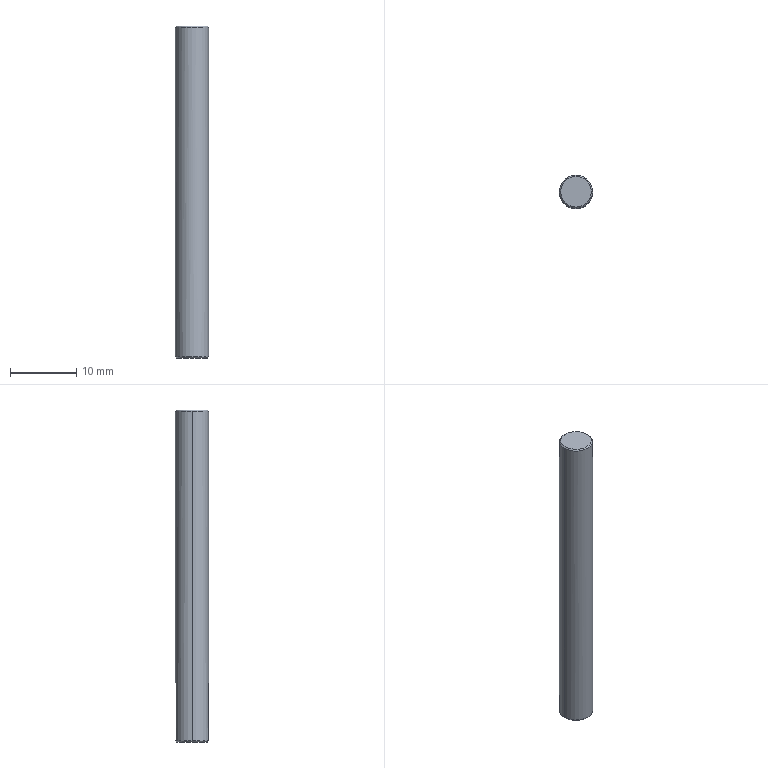Part | SolidWorks | features BaseBody 1 | 1 solid | 8 faces | box 5 x 5 x 50 mm | volume 981.136 mm3 | cone 4 | cylinder 2 | plane 2 | commonest cylinder face diameters 5 x2
STEP:
#1=CARTESIAN_POINT('',(2.5,0.,0.2));
#2=VERTEX_POINT('',#1);
#3=CARTESIAN_POINT('',(-2.5,0.,0.2));
#4=VERTEX_POINT('',#3);
#5=CARTESIAN_POINT('',(0.,0.,0.2));
#6=DIRECTION('',(0.,0.,1.));
#7=DIRECTION('',(1.,0.,0.));
#8=AXIS2_PLACEMENT_3D('',#5,#6,#7);
#9=CIRCLE('',#8,2.5);
#10=EDGE_CURVE('',#2,#4,#9,.T.);
#11=ORIENTED_EDGE('',*,*,#10,.T.);
#12=CARTESIAN_POINT('',(-2.5,0.,49.8));
#13=VERTEX_POINT('',#12);
#14=CARTESIAN_POINT('',(-2.5,0.,0.));
#15=DIRECTION('',(0.,0.,1.));
#16=VECTOR('',#15,1000.);
#17=LINE('',#14,#16);
#18=EDGE_CURVE('',#4,#13,#17,.T.);
#19=ORIENTED_EDGE('',*,*,#18,.T.);
#20=CARTESIAN_POINT('',(0.,2.5,49.8));
#21=VERTEX_POINT('',#20);
#22=CARTESIAN_POINT('',(0.,0.,49.8));
#23=DIRECTION('',(0.,0.,-1.));
#24=DIRECTION('',(1.,0.,0.));
#25=AXIS2_PLACEMENT_3D('',#22,#23,#24);
#26=CIRCLE('',#25,2.5);
#27=EDGE_CURVE('',#13,#21,#26,.T.);
#28=ORIENTED_EDGE('',*,*,#27,.T.);
#29=CARTESIAN_POINT('',(2.5,0.,49.8));
#30=VERTEX_POINT('',#29);
#31=CARTESIAN_POINT('',(0.,0.,49.8));
#32=DIRECTION('',(0.,0.,-1.));
#33=DIRECTION('',(1.,0.,0.));
#34=AXIS2_PLACEMENT_3D('',#31,#32,#33);
#35=CIRCLE('',#34,2.5);
#36=EDGE_CURVE('',#21,#30,#35,.T.);
#37=ORIENTED_EDGE('',*,*,#36,.T.);
#38=CARTESIAN_POINT('',(2.5,0.,0.));
#39=DIRECTION('',(0.,0.,1.));
#40=VECTOR('',#39,1000.);
#41=LINE('',#38,#40);
#42=EDGE_CURVE('',#2,#30,#41,.T.);
#43=ORIENTED_EDGE('',*,*,#42,.F.);
#44=EDGE_LOOP('',(#11,#19,#28,#37,#43));
#45=FACE_OUTER_BOUND('',#44,.T.);
#46=CARTESIAN_POINT('',(0.,0.,0.));
#47=DIRECTION('',(0.,0.,1.));
#48=DIRECTION('',(1.,0.,0.));
#49=AXIS2_PLACEMENT_3D('',#46,#47,#48);
#50=CYLINDRICAL_SURFACE('',#49,2.5);
#51=ADVANCED_FACE('',(#45),#50,.T.);
#52=CARTESIAN_POINT('',(2.3,0.,0.));
#53=VERTEX_POINT('',#52);
#54=CARTESIAN_POINT('',(-2.3,0.,0.));
#55=VERTEX_POINT('',#54);
#56=CARTESIAN_POINT('',(0.,0.,0.));
#57=DIRECTION('',(0.,0.,1.));
#58=DIRECTION('',(1.,0.,0.));
#59=AXIS2_PLACEMENT_3D('',#56,#57,#58);
#60=CIRCLE('',#59,2.3);
#61=EDGE_CURVE('',#53,#55,#60,.T.);
#62=ORIENTED_EDGE('',*,*,#61,.T.);
#63=CARTESIAN_POINT('',(-2.5,0.,0.2));
#64=DIRECTION('',(-0.7071,0.,0.7071));
#65=VECTOR('',#64,1000.);
#66=LINE('',#63,#65);
#67=EDGE_CURVE('',#55,#4,#66,.T.);
#68=ORIENTED_EDGE('',*,*,#67,.T.);
#69=ORIENTED_EDGE('',*,*,#10,.F.);
#70=CARTESIAN_POINT('',(2.5,0.,0.2));
#71=DIRECTION('',(0.7071,0.,0.7071));
#72=VECTOR('',#71,1000.);
#73=LINE('',#70,#72);
#74=EDGE_CURVE('',#53,#2,#73,.T.);
#75=ORIENTED_EDGE('',*,*,#74,.F.);
#76=EDGE_LOOP('',(#62,#68,#69,#75));
#77=FACE_OUTER_BOUND('',#76,.T.);
#78=CARTESIAN_POINT('',(0.,0.,0.2));
#79=DIRECTION('',(0.,0.,1.));
#80=DIRECTION('',(1.,0.,0.));
#81=AXIS2_PLACEMENT_3D('',#78,#79,#80);
#82=CONICAL_SURFACE('',#81,2.5,0.7854);
#83=ADVANCED_FACE('',(#77),#82,.T.);
#84=CARTESIAN_POINT('',(0.,2.3,50.));
#85=VERTEX_POINT('',#84);
#86=CARTESIAN_POINT('',(0.,-2.3,50.));
#87=VERTEX_POINT('',#86);
#88=CARTESIAN_POINT('',(0.,0.,50.));
#89=DIRECTION('',(0.,0.,-1.));
#90=DIRECTION('',(0.,1.,0.));
#91=AXIS2_PLACEMENT_3D('',#88,#89,#90);
#92=CIRCLE('',#91,2.3);
#93=EDGE_CURVE('',#85,#87,#92,.T.);
#94=ORIENTED_EDGE('',*,*,#93,.T.);
#95=CARTESIAN_POINT('',(0.,-2.5,49.8));
#96=VERTEX_POINT('',#95);
#97=CARTESIAN_POINT('',(0.,-2.5,49.8));
#98=DIRECTION('',(0.,-0.7071,-0.7071));
#99=VECTOR('',#98,1000.);
#100=LINE('',#97,#99);
#101=EDGE_CURVE('',#87,#96,#100,.T.);
#102=ORIENTED_EDGE('',*,*,#101,.T.);
#103=CARTESIAN_POINT('',(0.,0.,49.8));
#104=DIRECTION('',(0.,0.,-1.));
#105=DIRECTION('',(1.,0.,0.));
#106=AXIS2_PLACEMENT_3D('',#103,#104,#105);
#107=CIRCLE('',#106,2.5);
#108=EDGE_CURVE('',#30,#96,#107,.T.);
#109=ORIENTED_EDGE('',*,*,#108,.F.);
#110=ORIENTED_EDGE('',*,*,#36,.F.);
#111=CARTESIAN_POINT('',(0.,2.5,49.8));
#112=DIRECTION('',(0.,0.7071,-0.7071));
#113=VECTOR('',#112,1000.);
#114=LINE('',#111,#113);
#115=EDGE_CURVE('',#85,#21,#114,.T.);
#116=ORIENTED_EDGE('',*,*,#115,.F.);
#117=EDGE_LOOP('',(#94,#102,#109,#110,#116));
#118=FACE_OUTER_BOUND('',#117,.T.);
#119=CARTESIAN_POINT('',(0.,0.,49.8));
#120=DIRECTION('',(0.,0.,-1.));
#121=DIRECTION('',(0.,1.,0.));
#122=AXIS2_PLACEMENT_3D('',#119,#120,#121);
#123=CONICAL_SURFACE('',#122,2.5,0.7854);
#124=ADVANCED_FACE('',(#118),#123,.T.);
#125=ORIENTED_EDGE('',*,*,#18,.F.);
#126=CARTESIAN_POINT('',(0.,0.,0.2));
#127=DIRECTION('',(0.,0.,1.));
#128=DIRECTION('',(1.,0.,0.));
#129=AXIS2_PLACEMENT_3D('',#126,#127,#128);
#130=CIRCLE('',#129,2.5);
#131=EDGE_CURVE('',#4,#2,#130,.T.);
#132=ORIENTED_EDGE('',*,*,#131,.T.);
#133=ORIENTED_EDGE('',*,*,#42,.T.);
#134=ORIENTED_EDGE('',*,*,#108,.T.);
#135=CARTESIAN_POINT('',(0.,0.,49.8));
#136=DIRECTION('',(0.,0.,-1.));
#137=DIRECTION('',(1.,0.,0.));
#138=AXIS2_PLACEMENT_3D('',#135,#136,#137);
#139=CIRCLE('',#138,2.5);
#140=EDGE_CURVE('',#96,#13,#139,.T.);
#141=ORIENTED_EDGE('',*,*,#140,.T.);
#142=EDGE_LOOP('',(#125,#132,#133,#134,#141));
#143=FACE_OUTER_BOUND('',#142,.T.);
#144=CARTESIAN_POINT('',(0.,0.,0.));
#145=DIRECTION('',(0.,0.,1.));
#146=DIRECTION('',(1.,0.,0.));
#147=AXIS2_PLACEMENT_3D('',#144,#145,#146);
#148=CYLINDRICAL_SURFACE('',#147,2.5);
#149=ADVANCED_FACE('',(#143),#148,.T.);
#150=ORIENTED_EDGE('',*,*,#67,.F.);
#151=CARTESIAN_POINT('',(0.,0.,0.));
#152=DIRECTION('',(0.,0.,1.));
#153=DIRECTION('',(1.,0.,0.));
#154=AXIS2_PLACEMENT_3D('',#151,#152,#153);
#155=CIRCLE('',#154,2.3);
#156=EDGE_CURVE('',#55,#53,#155,.T.);
#157=ORIENTED_EDGE('',*,*,#156,.T.);
#158=ORIENTED_EDGE('',*,*,#74,.T.);
#159=ORIENTED_EDGE('',*,*,#131,.F.);
#160=EDGE_LOOP('',(#150,#157,#158,#159));
#161=FACE_OUTER_BOUND('',#160,.T.);
#162=CARTESIAN_POINT('',(0.,0.,0.2));
#163=DIRECTION('',(0.,0.,1.));
#164=DIRECTION('',(1.,0.,0.));
#165=AXIS2_PLACEMENT_3D('',#162,#163,#164);
#166=CONICAL_SURFACE('',#165,2.5,0.7854);
#167=ADVANCED_FACE('',(#161),#166,.T.);
#168=ORIENTED_EDGE('',*,*,#101,.F.);
#169=CARTESIAN_POINT('',(0.,0.,50.));
#170=DIRECTION('',(0.,0.,-1.));
#171=DIRECTION('',(0.,1.,0.));
#172=AXIS2_PLACEMENT_3D('',#169,#170,#171);
#173=CIRCLE('',#172,2.3);
#174=EDGE_CURVE('',#87,#85,#173,.T.);
#175=ORIENTED_EDGE('',*,*,#174,.T.);
#176=ORIENTED_EDGE('',*,*,#115,.T.);
#177=ORIENTED_EDGE('',*,*,#27,.F.);
#178=ORIENTED_EDGE('',*,*,#140,.F.);
#179=EDGE_LOOP('',(#168,#175,#176,#177,#178));
#180=FACE_OUTER_BOUND('',#179,.T.);
#181=CARTESIAN_POINT('',(0.,0.,49.8));
#182=DIRECTION('',(0.,0.,-1.));
#183=DIRECTION('',(0.,1.,0.));
#184=AXIS2_PLACEMENT_3D('',#181,#182,#183);
#185=CONICAL_SURFACE('',#184,2.5,0.7854);
#186=ADVANCED_FACE('',(#180),#185,.T.);
#187=ORIENTED_EDGE('',*,*,#61,.F.);
#188=ORIENTED_EDGE('',*,*,#156,.F.);
#189=EDGE_LOOP('',(#187,#188));
#190=FACE_OUTER_BOUND('',#189,.T.);
#191=CARTESIAN_POINT('',(0.,0.,0.));
#192=DIRECTION('',(0.,0.,-1.));
#193=DIRECTION('',(-1.,0.,0.));
#194=AXIS2_PLACEMENT_3D('',#191,#192,#193);
#195=PLANE('',#194);
#196=ADVANCED_FACE('',(#190),#195,.T.);
#197=ORIENTED_EDGE('',*,*,#93,.F.);
#198=ORIENTED_EDGE('',*,*,#174,.F.);
#199=EDGE_LOOP('',(#197,#198));
#200=FACE_OUTER_BOUND('',#199,.T.);
#201=CARTESIAN_POINT('',(0.,0.,50.));
#202=DIRECTION('',(0.,0.,-1.));
#203=DIRECTION('',(-1.,0.,0.));
#204=AXIS2_PLACEMENT_3D('',#201,#202,#203);
#205=PLANE('',#204);
#206=ADVANCED_FACE('',(#200),#205,.F.);
#207=CLOSED_SHELL('',(#51,#83,#124,#149,#167,#186,#196,#206));
#208=MANIFOLD_SOLID_BREP('',#207);
#209=CARTESIAN_POINT('',(0.,0.,0.));
#210=DIRECTION('',(0.,0.,1.));
#211=DIRECTION('',(1.,0.,0.));
#212=AXIS2_PLACEMENT_3D('',#209,#210,#211);
#213=(LENGTH_UNIT()NAMED_UNIT(*)SI_UNIT(.MILLI.,.METRE.));
#214=UNCERTAINTY_MEASURE_WITH_UNIT(LENGTH_MEASURE(0.00001),#213,'','');
#215=(NAMED_UNIT(*)PLANE_ANGLE_UNIT()SI_UNIT($,.RADIAN.));
#216=(NAMED_UNIT(*)SI_UNIT($,.STERADIAN.)SOLID_ANGLE_UNIT());
#217=(GEOMETRIC_REPRESENTATION_CONTEXT(3)GLOBAL_UNCERTAINTY_ASSIGNED_CONTEXT((#214))GLOBAL_UNIT_ASSIGNED_CONTEXT((#213,#215,#216))REPRESENTATION_CONTEXT('',''));
#218=ADVANCED_BREP_SHAPE_REPRESENTATION('',(#208,#212),#217);